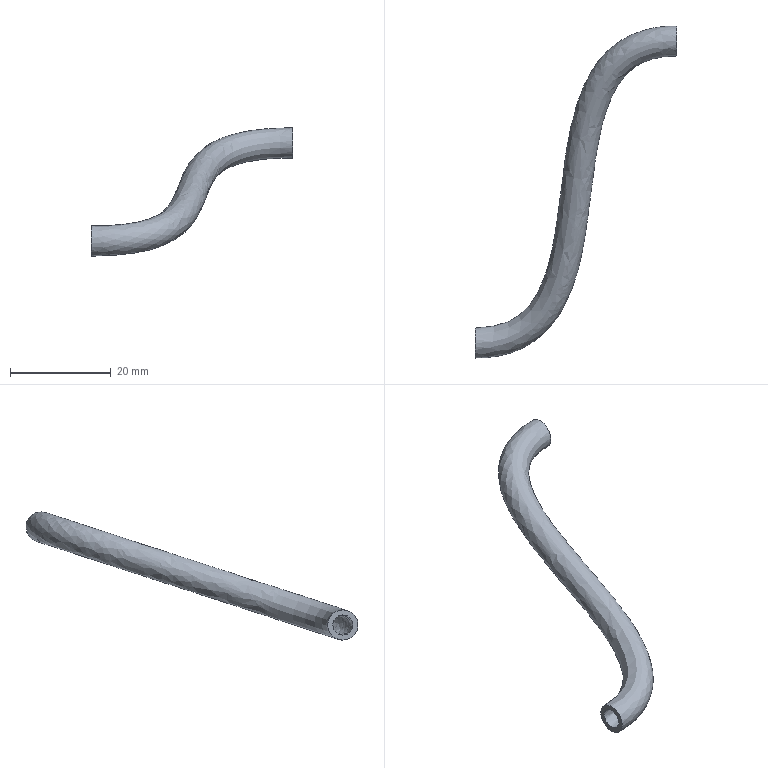Part | NX | features solid 2 | 1 solid | 4 faces | box 40.037 x 66.003 x 25.5 mm | volume 1311 mm3 | plane 2 | spline 2